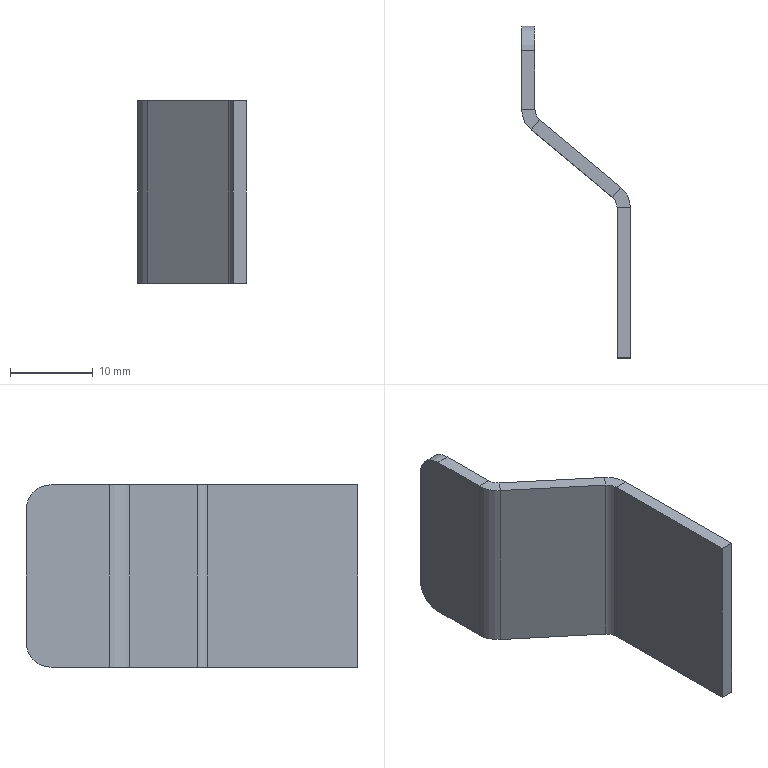Part | SolidWorks | features BreakCorner 1, FlatPattern 1, SMBaseFlange 1, SheetMetal 1 | 1 solid | 24 faces | box 13.1 x 40 x 22 mm | volume 1581 mm3 | plane 18 | cylinder 6 | commonest cylinder face diameters 3.2 x2 6 x2 6.4 x2
STEP:
#1=CARTESIAN_POINT('',(0.,18.103,11.));
#2=VERTEX_POINT('',#1);
#3=CARTESIAN_POINT('',(-1.6,18.103,11.));
#4=VERTEX_POINT('',#3);
#5=CARTESIAN_POINT('',(0.,18.103,11.));
#6=DIRECTION('',(-1.,0.,0.));
#7=VECTOR('',#6,1000.);
#8=LINE('',#5,#7);
#9=EDGE_CURVE('',#2,#4,#8,.T.);
#10=ORIENTED_EDGE('',*,*,#9,.F.);
#11=CARTESIAN_POINT('',(-1.149,20.559,11.));
#12=VERTEX_POINT('',#11);
#13=CARTESIAN_POINT('',(-3.2,18.103,11.));
#14=DIRECTION('',(0.,0.,1.));
#15=DIRECTION('',(-1.,0.,0.));
#16=AXIS2_PLACEMENT_3D('',#13,#14,#15);
#17=CIRCLE('',#16,3.2);
#18=EDGE_CURVE('',#2,#12,#17,.T.);
#19=ORIENTED_EDGE('',*,*,#18,.T.);
#20=CARTESIAN_POINT('',(-2.175,19.331,11.));
#21=VERTEX_POINT('',#20);
#22=CARTESIAN_POINT('',(-2.175,19.331,11.));
#23=DIRECTION('',(0.6408,0.7677,0.));
#24=VECTOR('',#23,1000.);
#25=LINE('',#22,#24);
#26=EDGE_CURVE('',#21,#12,#25,.T.);
#27=ORIENTED_EDGE('',*,*,#26,.F.);
#28=CARTESIAN_POINT('',(-3.2,18.103,11.));
#29=DIRECTION('',(0.,0.,1.));
#30=DIRECTION('',(1.,0.,0.));
#31=AXIS2_PLACEMENT_3D('',#28,#29,#30);
#32=CIRCLE('',#31,1.6);
#33=EDGE_CURVE('',#4,#21,#32,.T.);
#34=ORIENTED_EDGE('',*,*,#33,.F.);
#35=EDGE_LOOP('',(#10,#19,#27,#34));
#36=FACE_OUTER_BOUND('',#35,.T.);
#37=CARTESIAN_POINT('',(0.,18.103,11.));
#38=DIRECTION('',(0.,0.,1.));
#39=DIRECTION('',(1.,0.,0.));
#40=AXIS2_PLACEMENT_3D('',#37,#38,#39);
#41=PLANE('',#40);
#42=ADVANCED_FACE('',(#36),#41,.T.);
#43=CARTESIAN_POINT('',(0.,0.,11.));
#44=VERTEX_POINT('',#43);
#45=CARTESIAN_POINT('',(0.,0.,11.));
#46=DIRECTION('',(0.,1.,0.));
#47=VECTOR('',#46,1000.);
#48=LINE('',#45,#47);
#49=EDGE_CURVE('',#44,#2,#48,.T.);
#50=ORIENTED_EDGE('',*,*,#49,.T.);
#51=ORIENTED_EDGE('',*,*,#9,.T.);
#52=CARTESIAN_POINT('',(-1.6,0.,11.));
#53=VERTEX_POINT('',#52);
#54=CARTESIAN_POINT('',(-1.6,0.,11.));
#55=DIRECTION('',(0.,1.,0.));
#56=VECTOR('',#55,1000.);
#57=LINE('',#54,#56);
#58=EDGE_CURVE('',#53,#4,#57,.T.);
#59=ORIENTED_EDGE('',*,*,#58,.F.);
#60=CARTESIAN_POINT('',(0.,0.,11.));
#61=DIRECTION('',(-1.,0.,0.));
#62=VECTOR('',#61,1000.);
#63=LINE('',#60,#62);
#64=EDGE_CURVE('',#44,#53,#63,.T.);
#65=ORIENTED_EDGE('',*,*,#64,.F.);
#66=EDGE_LOOP('',(#50,#51,#59,#65));
#67=FACE_OUTER_BOUND('',#66,.T.);
#68=CARTESIAN_POINT('',(-2.175,19.331,11.));
#69=DIRECTION('',(0.,0.,1.));
#70=DIRECTION('',(1.,0.,0.));
#71=AXIS2_PLACEMENT_3D('',#68,#69,#70);
#72=PLANE('',#71);
#73=ADVANCED_FACE('',(#67),#72,.T.);
#74=CARTESIAN_POINT('',(-1.149,20.559,-11.));
#75=VERTEX_POINT('',#74);
#76=CARTESIAN_POINT('',(-2.175,19.331,-11.));
#77=VERTEX_POINT('',#76);
#78=CARTESIAN_POINT('',(-1.149,20.559,-11.));
#79=DIRECTION('',(-0.6408,-0.7677,0.));
#80=VECTOR('',#79,1000.);
#81=LINE('',#78,#80);
#82=EDGE_CURVE('',#75,#77,#81,.T.);
#83=ORIENTED_EDGE('',*,*,#82,.F.);
#84=CARTESIAN_POINT('',(0.,18.103,-11.));
#85=VERTEX_POINT('',#84);
#86=CARTESIAN_POINT('',(-3.2,18.103,-11.));
#87=DIRECTION('',(0.,0.,1.));
#88=DIRECTION('',(-1.,0.,0.));
#89=AXIS2_PLACEMENT_3D('',#86,#87,#88);
#90=CIRCLE('',#89,3.2);
#91=EDGE_CURVE('',#85,#75,#90,.T.);
#92=ORIENTED_EDGE('',*,*,#91,.F.);
#93=CARTESIAN_POINT('',(-1.6,18.103,-11.));
#94=VERTEX_POINT('',#93);
#95=CARTESIAN_POINT('',(-1.6,18.103,-11.));
#96=DIRECTION('',(1.,0.,0.));
#97=VECTOR('',#96,1000.);
#98=LINE('',#95,#97);
#99=EDGE_CURVE('',#94,#85,#98,.T.);
#100=ORIENTED_EDGE('',*,*,#99,.F.);
#101=CARTESIAN_POINT('',(-3.2,18.103,-11.));
#102=DIRECTION('',(0.,0.,1.));
#103=DIRECTION('',(1.,0.,0.));
#104=AXIS2_PLACEMENT_3D('',#101,#102,#103);
#105=CIRCLE('',#104,1.6);
#106=EDGE_CURVE('',#94,#77,#105,.T.);
#107=ORIENTED_EDGE('',*,*,#106,.T.);
#108=EDGE_LOOP('',(#83,#92,#100,#107));
#109=FACE_OUTER_BOUND('',#108,.T.);
#110=CARTESIAN_POINT('',(-1.149,20.559,-11.));
#111=DIRECTION('',(0.,0.,-1.));
#112=DIRECTION('',(-1.,0.,0.));
#113=AXIS2_PLACEMENT_3D('',#110,#111,#112);
#114=PLANE('',#113);
#115=ADVANCED_FACE('',(#109),#114,.T.);
#116=CARTESIAN_POINT('',(-10.925,28.72,-11.));
#117=VERTEX_POINT('',#116);
#118=CARTESIAN_POINT('',(0.,19.6,-11.));
#119=DIRECTION('',(-0.7677,0.6408,0.));
#120=VECTOR('',#119,1000.);
#121=LINE('',#118,#120);
#122=EDGE_CURVE('',#75,#117,#121,.T.);
#123=ORIENTED_EDGE('',*,*,#122,.F.);
#124=ORIENTED_EDGE('',*,*,#82,.T.);
#125=CARTESIAN_POINT('',(-11.951,27.492,-11.));
#126=VERTEX_POINT('',#125);
#127=CARTESIAN_POINT('',(-1.025,18.372,-11.));
#128=DIRECTION('',(-0.7677,0.6408,0.));
#129=VECTOR('',#128,1000.);
#130=LINE('',#127,#129);
#131=EDGE_CURVE('',#77,#126,#130,.T.);
#132=ORIENTED_EDGE('',*,*,#131,.T.);
#133=CARTESIAN_POINT('',(-11.951,27.492,-11.));
#134=DIRECTION('',(0.6408,0.7677,0.));
#135=VECTOR('',#134,1000.);
#136=LINE('',#133,#135);
#137=EDGE_CURVE('',#126,#117,#136,.T.);
#138=ORIENTED_EDGE('',*,*,#137,.T.);
#139=EDGE_LOOP('',(#123,#124,#132,#138));
#140=FACE_OUTER_BOUND('',#139,.T.);
#141=CARTESIAN_POINT('',(-1.6,18.103,-11.));
#142=DIRECTION('',(0.,0.,-1.));
#143=DIRECTION('',(-1.,0.,0.));
#144=AXIS2_PLACEMENT_3D('',#141,#142,#143);
#145=PLANE('',#144);
#146=ADVANCED_FACE('',(#140),#145,.T.);
#147=CARTESIAN_POINT('',(-10.925,28.72,11.));
#148=VERTEX_POINT('',#147);
#149=CARTESIAN_POINT('',(-11.951,27.492,11.));
#150=VERTEX_POINT('',#149);
#151=CARTESIAN_POINT('',(-10.925,28.72,11.));
#152=DIRECTION('',(-0.6408,-0.7677,0.));
#153=VECTOR('',#152,1000.);
#154=LINE('',#151,#153);
#155=EDGE_CURVE('',#148,#150,#154,.T.);
#156=ORIENTED_EDGE('',*,*,#155,.F.);
#157=CARTESIAN_POINT('',(-11.5,29.949,11.));
#158=VERTEX_POINT('',#157);
#159=CARTESIAN_POINT('',(-9.9,29.949,11.));
#160=DIRECTION('',(0.,0.,-1.));
#161=DIRECTION('',(1.,0.,0.));
#162=AXIS2_PLACEMENT_3D('',#159,#160,#161);
#163=CIRCLE('',#162,1.6);
#164=EDGE_CURVE('',#148,#158,#163,.T.);
#165=ORIENTED_EDGE('',*,*,#164,.T.);
#166=CARTESIAN_POINT('',(-13.1,29.949,11.));
#167=VERTEX_POINT('',#166);
#168=CARTESIAN_POINT('',(-13.1,29.949,11.));
#169=DIRECTION('',(1.,0.,0.));
#170=VECTOR('',#169,1000.);
#171=LINE('',#168,#170);
#172=EDGE_CURVE('',#167,#158,#171,.T.);
#173=ORIENTED_EDGE('',*,*,#172,.F.);
#174=CARTESIAN_POINT('',(-9.9,29.949,11.));
#175=DIRECTION('',(0.,0.,-1.));
#176=DIRECTION('',(1.,0.,0.));
#177=AXIS2_PLACEMENT_3D('',#174,#175,#176);
#178=CIRCLE('',#177,3.2);
#179=EDGE_CURVE('',#150,#167,#178,.T.);
#180=ORIENTED_EDGE('',*,*,#179,.F.);
#181=EDGE_LOOP('',(#156,#165,#173,#180));
#182=FACE_OUTER_BOUND('',#181,.T.);
#183=CARTESIAN_POINT('',(-10.925,28.72,11.));
#184=DIRECTION('',(0.,0.,1.));
#185=DIRECTION('',(1.,0.,0.));
#186=AXIS2_PLACEMENT_3D('',#183,#184,#185);
#187=PLANE('',#186);
#188=ADVANCED_FACE('',(#182),#187,.T.);
#189=CARTESIAN_POINT('',(0.,19.6,11.));
#190=DIRECTION('',(-0.7677,0.6408,0.));
#191=VECTOR('',#190,1000.);
#192=LINE('',#189,#191);
#193=EDGE_CURVE('',#12,#148,#192,.T.);
#194=ORIENTED_EDGE('',*,*,#193,.T.);
#195=ORIENTED_EDGE('',*,*,#155,.T.);
#196=CARTESIAN_POINT('',(-1.025,18.372,11.));
#197=DIRECTION('',(-0.7677,0.6408,0.));
#198=VECTOR('',#197,1000.);
#199=LINE('',#196,#198);
#200=EDGE_CURVE('',#21,#150,#199,.T.);
#201=ORIENTED_EDGE('',*,*,#200,.F.);
#202=ORIENTED_EDGE('',*,*,#26,.T.);
#203=EDGE_LOOP('',(#194,#195,#201,#202));
#204=FACE_OUTER_BOUND('',#203,.T.);
#205=CARTESIAN_POINT('',(-13.1,29.949,11.));
#206=DIRECTION('',(0.,0.,1.));
#207=DIRECTION('',(1.,0.,0.));
#208=AXIS2_PLACEMENT_3D('',#205,#206,#207);
#209=PLANE('',#208);
#210=ADVANCED_FACE('',(#204),#209,.T.);
#211=CARTESIAN_POINT('',(-11.5,29.949,-11.));
#212=VERTEX_POINT('',#211);
#213=CARTESIAN_POINT('',(-13.1,29.949,-11.));
#214=VERTEX_POINT('',#213);
#215=CARTESIAN_POINT('',(-11.5,29.949,-11.));
#216=DIRECTION('',(-1.,0.,0.));
#217=VECTOR('',#216,1000.);
#218=LINE('',#215,#217);
#219=EDGE_CURVE('',#212,#214,#218,.T.);
#220=ORIENTED_EDGE('',*,*,#219,.F.);
#221=CARTESIAN_POINT('',(-9.9,29.949,-11.));
#222=DIRECTION('',(0.,0.,-1.));
#223=DIRECTION('',(1.,0.,0.));
#224=AXIS2_PLACEMENT_3D('',#221,#222,#223);
#225=CIRCLE('',#224,1.6);
#226=EDGE_CURVE('',#117,#212,#225,.T.);
#227=ORIENTED_EDGE('',*,*,#226,.F.);
#228=ORIENTED_EDGE('',*,*,#137,.F.);
#229=CARTESIAN_POINT('',(-9.9,29.949,-11.));
#230=DIRECTION('',(0.,0.,-1.));
#231=DIRECTION('',(1.,0.,0.));
#232=AXIS2_PLACEMENT_3D('',#229,#230,#231);
#233=CIRCLE('',#232,3.2);
#234=EDGE_CURVE('',#126,#214,#233,.T.);
#235=ORIENTED_EDGE('',*,*,#234,.T.);
#236=EDGE_LOOP('',(#220,#227,#228,#235));
#237=FACE_OUTER_BOUND('',#236,.T.);
#238=CARTESIAN_POINT('',(-11.5,29.949,-11.));
#239=DIRECTION('',(0.,0.,-1.));
#240=DIRECTION('',(-1.,0.,0.));
#241=AXIS2_PLACEMENT_3D('',#238,#239,#240);
#242=PLANE('',#241);
#243=ADVANCED_FACE('',(#237),#242,.T.);
#244=CARTESIAN_POINT('',(-13.1,37.,-11.));
#245=VERTEX_POINT('',#244);
#246=CARTESIAN_POINT('',(-13.1,29.2,-11.));
#247=DIRECTION('',(0.,1.,0.));
#248=VECTOR('',#247,1000.);
#249=LINE('',#246,#248);
#250=EDGE_CURVE('',#214,#245,#249,.T.);
#251=ORIENTED_EDGE('',*,*,#250,.T.);
#252=CARTESIAN_POINT('',(-11.5,37.,-11.));
#253=VERTEX_POINT('',#252);
#254=CARTESIAN_POINT('',(-11.951,37.,-11.));
#255=DIRECTION('',(1.,0.,0.));
#256=VECTOR('',#255,1000.);
#257=LINE('',#254,#256);
#258=EDGE_CURVE('',#245,#253,#257,.T.);
#259=ORIENTED_EDGE('',*,*,#258,.T.);
#260=CARTESIAN_POINT('',(-11.5,29.2,-11.));
#261=DIRECTION('',(0.,1.,0.));
#262=VECTOR('',#261,1000.);
#263=LINE('',#260,#262);
#264=EDGE_CURVE('',#212,#253,#263,.T.);
#265=ORIENTED_EDGE('',*,*,#264,.F.);
#266=ORIENTED_EDGE('',*,*,#219,.T.);
#267=EDGE_LOOP('',(#251,#259,#265,#266));
#268=FACE_OUTER_BOUND('',#267,.T.);
#269=CARTESIAN_POINT('',(-11.951,27.492,-11.));
#270=DIRECTION('',(0.,0.,-1.));
#271=DIRECTION('',(-1.,0.,0.));
#272=AXIS2_PLACEMENT_3D('',#269,#270,#271);
#273=PLANE('',#272);
#274=ADVANCED_FACE('',(#268),#273,.T.);
#275=ORIENTED_EDGE('',*,*,#264,.T.);
#276=CARTESIAN_POINT('',(-11.5,40.,-8.));
#277=VERTEX_POINT('',#276);
#278=CARTESIAN_POINT('',(-11.5,37.,-8.));
#279=DIRECTION('',(1.,0.,0.));
#280=DIRECTION('',(0.,0.,1.));
#281=AXIS2_PLACEMENT_3D('',#278,#279,#280);
#282=CIRCLE('',#281,3.);
#283=EDGE_CURVE('',#253,#277,#282,.T.);
#284=ORIENTED_EDGE('',*,*,#283,.T.);
#285=CARTESIAN_POINT('',(-11.5,40.,8.));
#286=VERTEX_POINT('',#285);
#287=CARTESIAN_POINT('',(-11.5,40.,11.));
#288=DIRECTION('',(0.,0.,-1.));
#289=VECTOR('',#288,1000.);
#290=LINE('',#287,#289);
#291=EDGE_CURVE('',#286,#277,#290,.T.);
#292=ORIENTED_EDGE('',*,*,#291,.F.);
#293=CARTESIAN_POINT('',(-11.5,37.,11.));
#294=VERTEX_POINT('',#293);
#295=CARTESIAN_POINT('',(-11.5,37.,8.));
#296=DIRECTION('',(1.,0.,0.));
#297=DIRECTION('',(0.,0.,1.));
#298=AXIS2_PLACEMENT_3D('',#295,#296,#297);
#299=CIRCLE('',#298,3.);
#300=EDGE_CURVE('',#286,#294,#299,.T.);
#301=ORIENTED_EDGE('',*,*,#300,.T.);
#302=CARTESIAN_POINT('',(-11.5,29.2,11.));
#303=DIRECTION('',(0.,1.,0.));
#304=VECTOR('',#303,1000.);
#305=LINE('',#302,#304);
#306=EDGE_CURVE('',#158,#294,#305,.T.);
#307=ORIENTED_EDGE('',*,*,#306,.F.);
#308=CARTESIAN_POINT('',(-11.5,29.949,11.));
#309=DIRECTION('',(0.,0.,-1.));
#310=VECTOR('',#309,1000.);
#311=LINE('',#308,#310);
#312=EDGE_CURVE('',#158,#212,#311,.T.);
#313=ORIENTED_EDGE('',*,*,#312,.T.);
#314=EDGE_LOOP('',(#275,#284,#292,#301,#307,#313));
#315=FACE_OUTER_BOUND('',#314,.T.);
#316=CARTESIAN_POINT('',(-11.5,29.2,11.));
#317=DIRECTION('',(-1.,0.,0.));
#318=DIRECTION('',(0.,0.,1.));
#319=AXIS2_PLACEMENT_3D('',#316,#317,#318);
#320=PLANE('',#319);
#321=ADVANCED_FACE('',(#315),#320,.F.);
#322=ORIENTED_EDGE('',*,*,#291,.T.);
#323=CARTESIAN_POINT('',(-13.1,40.,-8.));
#324=VERTEX_POINT('',#323);
#325=CARTESIAN_POINT('',(-13.1,40.,-8.));
#326=DIRECTION('',(-1.,0.,0.));
#327=VECTOR('',#326,1000.);
#328=LINE('',#325,#327);
#329=EDGE_CURVE('',#277,#324,#328,.T.);
#330=ORIENTED_EDGE('',*,*,#329,.T.);
#331=CARTESIAN_POINT('',(-13.1,40.,8.));
#332=VERTEX_POINT('',#331);
#333=CARTESIAN_POINT('',(-13.1,40.,11.));
#334=DIRECTION('',(0.,0.,-1.));
#335=VECTOR('',#334,1000.);
#336=LINE('',#333,#335);
#337=EDGE_CURVE('',#332,#324,#336,.T.);
#338=ORIENTED_EDGE('',*,*,#337,.F.);
#339=CARTESIAN_POINT('',(-13.1,40.,8.));
#340=DIRECTION('',(1.,0.,0.));
#341=VECTOR('',#340,1000.);
#342=LINE('',#339,#341);
#343=EDGE_CURVE('',#332,#286,#342,.T.);
#344=ORIENTED_EDGE('',*,*,#343,.T.);
#345=EDGE_LOOP('',(#322,#330,#338,#344));
#346=FACE_OUTER_BOUND('',#345,.T.);
#347=CARTESIAN_POINT('',(-13.1,40.,11.));
#348=DIRECTION('',(0.,1.,0.));
#349=DIRECTION('',(-1.,0.,0.));
#350=AXIS2_PLACEMENT_3D('',#347,#348,#349);
#351=PLANE('',#350);
#352=ADVANCED_FACE('',(#346),#351,.T.);
#353=ORIENTED_EDGE('',*,*,#337,.T.);
#354=CARTESIAN_POINT('',(-13.1,37.,-8.));
#355=DIRECTION('',(-1.,0.,0.));
#356=DIRECTION('',(0.,0.,1.));
#357=AXIS2_PLACEMENT_3D('',#354,#355,#356);
#358=CIRCLE('',#357,3.);
#359=EDGE_CURVE('',#324,#245,#358,.T.);
#360=ORIENTED_EDGE('',*,*,#359,.T.);
#361=ORIENTED_EDGE('',*,*,#250,.F.);
#362=CARTESIAN_POINT('',(-13.1,29.949,11.));
#363=DIRECTION('',(0.,0.,-1.));
#364=VECTOR('',#363,1000.);
#365=LINE('',#362,#364);
#366=EDGE_CURVE('',#167,#214,#365,.T.);
#367=ORIENTED_EDGE('',*,*,#366,.F.);
#368=CARTESIAN_POINT('',(-13.1,37.,11.));
#369=VERTEX_POINT('',#368);
#370=CARTESIAN_POINT('',(-13.1,29.2,11.));
#371=DIRECTION('',(0.,1.,0.));
#372=VECTOR('',#371,1000.);
#373=LINE('',#370,#372);
#374=EDGE_CURVE('',#167,#369,#373,.T.);
#375=ORIENTED_EDGE('',*,*,#374,.T.);
#376=CARTESIAN_POINT('',(-13.1,37.,8.));
#377=DIRECTION('',(-1.,0.,0.));
#378=DIRECTION('',(0.,0.,1.));
#379=AXIS2_PLACEMENT_3D('',#376,#377,#378);
#380=CIRCLE('',#379,3.);
#381=EDGE_CURVE('',#369,#332,#380,.T.);
#382=ORIENTED_EDGE('',*,*,#381,.T.);
#383=EDGE_LOOP('',(#353,#360,#361,#367,#375,#382));
#384=FACE_OUTER_BOUND('',#383,.T.);
#385=CARTESIAN_POINT('',(-13.1,29.2,11.));
#386=DIRECTION('',(-1.,0.,0.));
#387=DIRECTION('',(0.,0.,1.));
#388=AXIS2_PLACEMENT_3D('',#385,#386,#387);
#389=PLANE('',#388);
#390=ADVANCED_FACE('',(#384),#389,.T.);
#391=ORIENTED_EDGE('',*,*,#234,.F.);
#392=CARTESIAN_POINT('',(-11.951,27.492,11.));
#393=DIRECTION('',(0.,0.,-1.));
#394=VECTOR('',#393,1000.);
#395=LINE('',#392,#394);
#396=EDGE_CURVE('',#150,#126,#395,.T.);
#397=ORIENTED_EDGE('',*,*,#396,.F.);
#398=ORIENTED_EDGE('',*,*,#179,.T.);
#399=ORIENTED_EDGE('',*,*,#366,.T.);
#400=EDGE_LOOP('',(#391,#397,#398,#399));
#401=FACE_OUTER_BOUND('',#400,.T.);
#402=CARTESIAN_POINT('',(-9.9,29.949,11.));
#403=DIRECTION('',(0.,0.,-1.));
#404=DIRECTION('',(-1.,0.,0.));
#405=AXIS2_PLACEMENT_3D('',#402,#403,#404);
#406=CYLINDRICAL_SURFACE('',#405,3.2);
#407=ADVANCED_FACE('',(#401),#406,.T.);
#408=ORIENTED_EDGE('',*,*,#131,.F.);
#409=CARTESIAN_POINT('',(-2.175,19.331,11.));
#410=DIRECTION('',(0.,0.,-1.));
#411=VECTOR('',#410,1000.);
#412=LINE('',#409,#411);
#413=EDGE_CURVE('',#21,#77,#412,.T.);
#414=ORIENTED_EDGE('',*,*,#413,.F.);
#415=ORIENTED_EDGE('',*,*,#200,.T.);
#416=ORIENTED_EDGE('',*,*,#396,.T.);
#417=EDGE_LOOP('',(#408,#414,#415,#416));
#418=FACE_OUTER_BOUND('',#417,.T.);
#419=CARTESIAN_POINT('',(-1.025,18.372,11.));
#420=DIRECTION('',(-0.6408,-0.7677,0.));
#421=DIRECTION('',(0.7677,-0.6408,0.));
#422=AXIS2_PLACEMENT_3D('',#419,#420,#421);
#423=PLANE('',#422);
#424=ADVANCED_FACE('',(#418),#423,.T.);
#425=ORIENTED_EDGE('',*,*,#106,.F.);
#426=CARTESIAN_POINT('',(-1.6,18.103,11.));
#427=DIRECTION('',(0.,0.,-1.));
#428=VECTOR('',#427,1000.);
#429=LINE('',#426,#428);
#430=EDGE_CURVE('',#4,#94,#429,.T.);
#431=ORIENTED_EDGE('',*,*,#430,.F.);
#432=ORIENTED_EDGE('',*,*,#33,.T.);
#433=ORIENTED_EDGE('',*,*,#413,.T.);
#434=EDGE_LOOP('',(#425,#431,#432,#433));
#435=FACE_OUTER_BOUND('',#434,.T.);
#436=CARTESIAN_POINT('',(-3.2,18.103,11.));
#437=DIRECTION('',(0.,0.,-1.));
#438=DIRECTION('',(-1.,0.,0.));
#439=AXIS2_PLACEMENT_3D('',#436,#437,#438);
#440=CYLINDRICAL_SURFACE('',#439,1.6);
#441=ADVANCED_FACE('',(#435),#440,.F.);
#442=CARTESIAN_POINT('',(-1.6,0.,-11.));
#443=VERTEX_POINT('',#442);
#444=CARTESIAN_POINT('',(-1.6,0.,-11.));
#445=DIRECTION('',(0.,1.,0.));
#446=VECTOR('',#445,1000.);
#447=LINE('',#444,#446);
#448=EDGE_CURVE('',#443,#94,#447,.T.);
#449=ORIENTED_EDGE('',*,*,#448,.F.);
#450=CARTESIAN_POINT('',(-1.6,0.,11.));
#451=DIRECTION('',(0.,0.,-1.));
#452=VECTOR('',#451,1000.);
#453=LINE('',#450,#452);
#454=EDGE_CURVE('',#53,#443,#453,.T.);
#455=ORIENTED_EDGE('',*,*,#454,.F.);
#456=ORIENTED_EDGE('',*,*,#58,.T.);
#457=ORIENTED_EDGE('',*,*,#430,.T.);
#458=EDGE_LOOP('',(#449,#455,#456,#457));
#459=FACE_OUTER_BOUND('',#458,.T.);
#460=CARTESIAN_POINT('',(-1.6,0.,11.));
#461=DIRECTION('',(-1.,0.,0.));
#462=DIRECTION('',(0.,0.,1.));
#463=AXIS2_PLACEMENT_3D('',#460,#461,#462);
#464=PLANE('',#463);
#465=ADVANCED_FACE('',(#459),#464,.T.);
#466=CARTESIAN_POINT('',(0.,0.,-11.));
#467=VERTEX_POINT('',#466);
#468=CARTESIAN_POINT('',(0.,0.,-11.));
#469=DIRECTION('',(-1.,0.,0.));
#470=VECTOR('',#469,1000.);
#471=LINE('',#468,#470);
#472=EDGE_CURVE('',#467,#443,#471,.T.);
#473=ORIENTED_EDGE('',*,*,#472,.F.);
#474=CARTESIAN_POINT('',(0.,0.,11.));
#475=DIRECTION('',(0.,0.,-1.));
#476=VECTOR('',#475,1000.);
#477=LINE('',#474,#476);
#478=EDGE_CURVE('',#44,#467,#477,.T.);
#479=ORIENTED_EDGE('',*,*,#478,.F.);
#480=ORIENTED_EDGE('',*,*,#64,.T.);
#481=ORIENTED_EDGE('',*,*,#454,.T.);
#482=EDGE_LOOP('',(#473,#479,#480,#481));
#483=FACE_OUTER_BOUND('',#482,.T.);
#484=CARTESIAN_POINT('',(0.,0.,11.));
#485=DIRECTION('',(0.,-1.,0.));
#486=DIRECTION('',(0.,0.,-1.));
#487=AXIS2_PLACEMENT_3D('',#484,#485,#486);
#488=PLANE('',#487);
#489=ADVANCED_FACE('',(#483),#488,.T.);
#490=CARTESIAN_POINT('',(0.,0.,-11.));
#491=DIRECTION('',(0.,1.,0.));
#492=VECTOR('',#491,1000.);
#493=LINE('',#490,#492);
#494=EDGE_CURVE('',#467,#85,#493,.T.);
#495=ORIENTED_EDGE('',*,*,#494,.T.);
#496=CARTESIAN_POINT('',(0.,18.103,11.));
#497=DIRECTION('',(0.,0.,-1.));
#498=VECTOR('',#497,1000.);
#499=LINE('',#496,#498);
#500=EDGE_CURVE('',#2,#85,#499,.T.);
#501=ORIENTED_EDGE('',*,*,#500,.F.);
#502=ORIENTED_EDGE('',*,*,#49,.F.);
#503=ORIENTED_EDGE('',*,*,#478,.T.);
#504=EDGE_LOOP('',(#495,#501,#502,#503));
#505=FACE_OUTER_BOUND('',#504,.T.);
#506=CARTESIAN_POINT('',(0.,0.,11.));
#507=DIRECTION('',(-1.,0.,0.));
#508=DIRECTION('',(0.,0.,1.));
#509=AXIS2_PLACEMENT_3D('',#506,#507,#508);
#510=PLANE('',#509);
#511=ADVANCED_FACE('',(#505),#510,.F.);
#512=ORIENTED_EDGE('',*,*,#91,.T.);
#513=CARTESIAN_POINT('',(-1.149,20.559,11.));
#514=DIRECTION('',(0.,0.,-1.));
#515=VECTOR('',#514,1000.);
#516=LINE('',#513,#515);
#517=EDGE_CURVE('',#12,#75,#516,.T.);
#518=ORIENTED_EDGE('',*,*,#517,.F.);
#519=ORIENTED_EDGE('',*,*,#18,.F.);
#520=ORIENTED_EDGE('',*,*,#500,.T.);
#521=EDGE_LOOP('',(#512,#518,#519,#520));
#522=FACE_OUTER_BOUND('',#521,.T.);
#523=CARTESIAN_POINT('',(-3.2,18.103,11.));
#524=DIRECTION('',(0.,0.,-1.));
#525=DIRECTION('',(-1.,0.,0.));
#526=AXIS2_PLACEMENT_3D('',#523,#524,#525);
#527=CYLINDRICAL_SURFACE('',#526,3.2);
#528=ADVANCED_FACE('',(#522),#527,.T.);
#529=ORIENTED_EDGE('',*,*,#122,.T.);
#530=CARTESIAN_POINT('',(-10.925,28.72,11.));
#531=DIRECTION('',(0.,0.,-1.));
#532=VECTOR('',#531,1000.);
#533=LINE('',#530,#532);
#534=EDGE_CURVE('',#148,#117,#533,.T.);
#535=ORIENTED_EDGE('',*,*,#534,.F.);
#536=ORIENTED_EDGE('',*,*,#193,.F.);
#537=ORIENTED_EDGE('',*,*,#517,.T.);
#538=EDGE_LOOP('',(#529,#535,#536,#537));
#539=FACE_OUTER_BOUND('',#538,.T.);
#540=CARTESIAN_POINT('',(0.,19.6,11.));
#541=DIRECTION('',(-0.6408,-0.7677,0.));
#542=DIRECTION('',(0.7677,-0.6408,0.));
#543=AXIS2_PLACEMENT_3D('',#540,#541,#542);
#544=PLANE('',#543);
#545=ADVANCED_FACE('',(#539),#544,.F.);
#546=ORIENTED_EDGE('',*,*,#226,.T.);
#547=ORIENTED_EDGE('',*,*,#312,.F.);
#548=ORIENTED_EDGE('',*,*,#164,.F.);
#549=ORIENTED_EDGE('',*,*,#534,.T.);
#550=EDGE_LOOP('',(#546,#547,#548,#549));
#551=FACE_OUTER_BOUND('',#550,.T.);
#552=CARTESIAN_POINT('',(-9.9,29.949,11.));
#553=DIRECTION('',(0.,0.,-1.));
#554=DIRECTION('',(-1.,0.,0.));
#555=AXIS2_PLACEMENT_3D('',#552,#553,#554);
#556=CYLINDRICAL_SURFACE('',#555,1.6);
#557=ADVANCED_FACE('',(#551),#556,.F.);
#558=ORIENTED_EDGE('',*,*,#306,.T.);
#559=CARTESIAN_POINT('',(-9.9,37.,11.));
#560=DIRECTION('',(-1.,0.,0.));
#561=VECTOR('',#560,1000.);
#562=LINE('',#559,#561);
#563=EDGE_CURVE('',#294,#369,#562,.T.);
#564=ORIENTED_EDGE('',*,*,#563,.T.);
#565=ORIENTED_EDGE('',*,*,#374,.F.);
#566=ORIENTED_EDGE('',*,*,#172,.T.);
#567=EDGE_LOOP('',(#558,#564,#565,#566));
#568=FACE_OUTER_BOUND('',#567,.T.);
#569=CARTESIAN_POINT('',(-9.9,29.949,11.));
#570=DIRECTION('',(0.,0.,1.));
#571=DIRECTION('',(1.,0.,0.));
#572=AXIS2_PLACEMENT_3D('',#569,#570,#571);
#573=PLANE('',#572);
#574=ADVANCED_FACE('',(#568),#573,.T.);
#575=ORIENTED_EDGE('',*,*,#448,.T.);
#576=ORIENTED_EDGE('',*,*,#99,.T.);
#577=ORIENTED_EDGE('',*,*,#494,.F.);
#578=ORIENTED_EDGE('',*,*,#472,.T.);
#579=EDGE_LOOP('',(#575,#576,#577,#578));
#580=FACE_OUTER_BOUND('',#579,.T.);
#581=CARTESIAN_POINT('',(-9.9,29.949,-11.));
#582=DIRECTION('',(0.,0.,1.));
#583=DIRECTION('',(1.,0.,0.));
#584=AXIS2_PLACEMENT_3D('',#581,#582,#583);
#585=PLANE('',#584);
#586=ADVANCED_FACE('',(#580),#585,.F.);
#587=ORIENTED_EDGE('',*,*,#359,.F.);
#588=ORIENTED_EDGE('',*,*,#329,.F.);
#589=ORIENTED_EDGE('',*,*,#283,.F.);
#590=ORIENTED_EDGE('',*,*,#258,.F.);
#591=EDGE_LOOP('',(#587,#588,#589,#590));
#592=FACE_OUTER_BOUND('',#591,.T.);
#593=CARTESIAN_POINT('',(-11.951,37.,-8.));
#594=DIRECTION('',(1.,0.,0.));
#595=DIRECTION('',(0.,1.,0.));
#596=AXIS2_PLACEMENT_3D('',#593,#594,#595);
#597=CYLINDRICAL_SURFACE('',#596,3.);
#598=ADVANCED_FACE('',(#592),#597,.T.);
#599=ORIENTED_EDGE('',*,*,#381,.F.);
#600=ORIENTED_EDGE('',*,*,#563,.F.);
#601=ORIENTED_EDGE('',*,*,#300,.F.);
#602=ORIENTED_EDGE('',*,*,#343,.F.);
#603=EDGE_LOOP('',(#599,#600,#601,#602));
#604=FACE_OUTER_BOUND('',#603,.T.);
#605=CARTESIAN_POINT('',(-13.1,37.,8.));
#606=DIRECTION('',(1.,0.,0.));
#607=DIRECTION('',(0.,1.,0.));
#608=AXIS2_PLACEMENT_3D('',#605,#606,#607);
#609=CYLINDRICAL_SURFACE('',#608,3.);
#610=ADVANCED_FACE('',(#604),#609,.T.);
#611=CLOSED_SHELL('',(#42,#73,#115,#146,#188,#210,#243,#274,#321,#352,#390,#407,#424,#441,#465,#489,#511,#528,#545,#557,#574,#586,#598,#610));
#612=MANIFOLD_SOLID_BREP('',#611);
#613=CARTESIAN_POINT('',(0.,0.,0.));
#614=DIRECTION('',(0.,0.,1.));
#615=DIRECTION('',(1.,0.,0.));
#616=AXIS2_PLACEMENT_3D('',#613,#614,#615);
#617=(LENGTH_UNIT()NAMED_UNIT(*)SI_UNIT(.MILLI.,.METRE.));
#618=UNCERTAINTY_MEASURE_WITH_UNIT(LENGTH_MEASURE(0.00001),#617,'','');
#619=(NAMED_UNIT(*)PLANE_ANGLE_UNIT()SI_UNIT($,.RADIAN.));
#620=(NAMED_UNIT(*)SI_UNIT($,.STERADIAN.)SOLID_ANGLE_UNIT());
#621=(GEOMETRIC_REPRESENTATION_CONTEXT(3)GLOBAL_UNCERTAINTY_ASSIGNED_CONTEXT((#618))GLOBAL_UNIT_ASSIGNED_CONTEXT((#617,#619,#620))REPRESENTATION_CONTEXT('',''));
#622=ADVANCED_BREP_SHAPE_REPRESENTATION('',(#612,#616),#621);